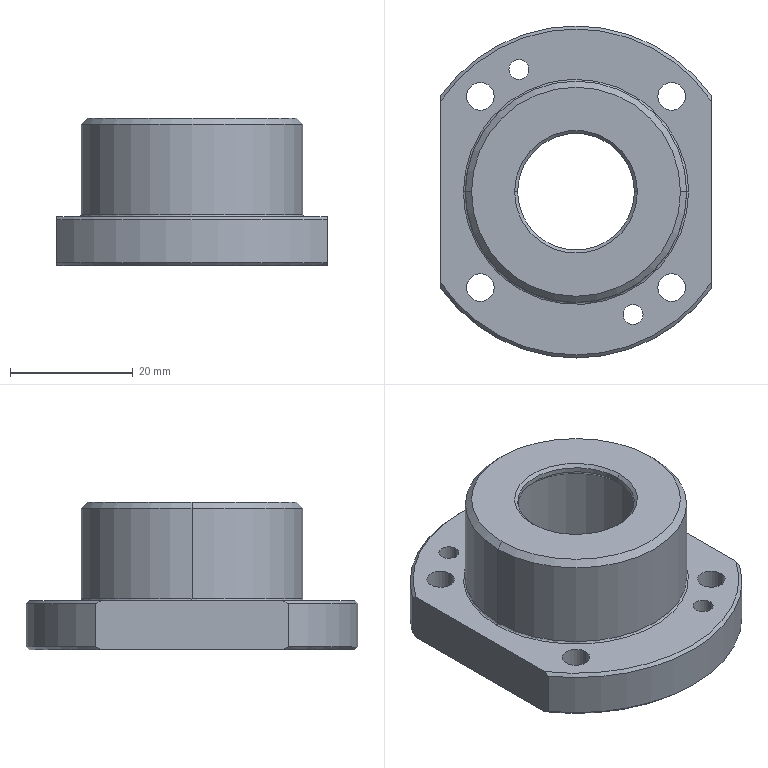Part | STEP file | 0230_Z_005_MRWZ12_1 | 1 solid | 62 faces | box 44 x 54 x 24 mm | volume 16765 mm3 | cylinder 32 | cone 16 | plane 12 | spline 2 | commonest cylinder face diameters 4.5 x8 8 x8 3.242 x4 19 x2 28 x2 30 x2